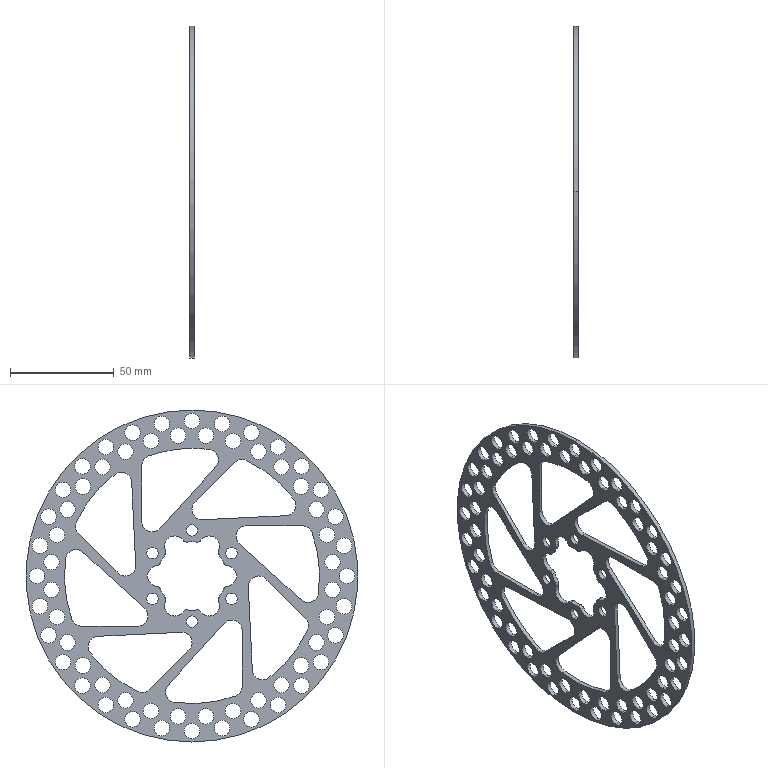Part | STEP file | Brake Disc | 1 solid | 228 faces | box 2 x 160 x 160 mm | volume 16953 mm3 | cylinder 210 | plane 18 | commonest cylinder face diameters 7.5 x128 10 x38 4 x14 5.5 x12 123 x9 33 x7